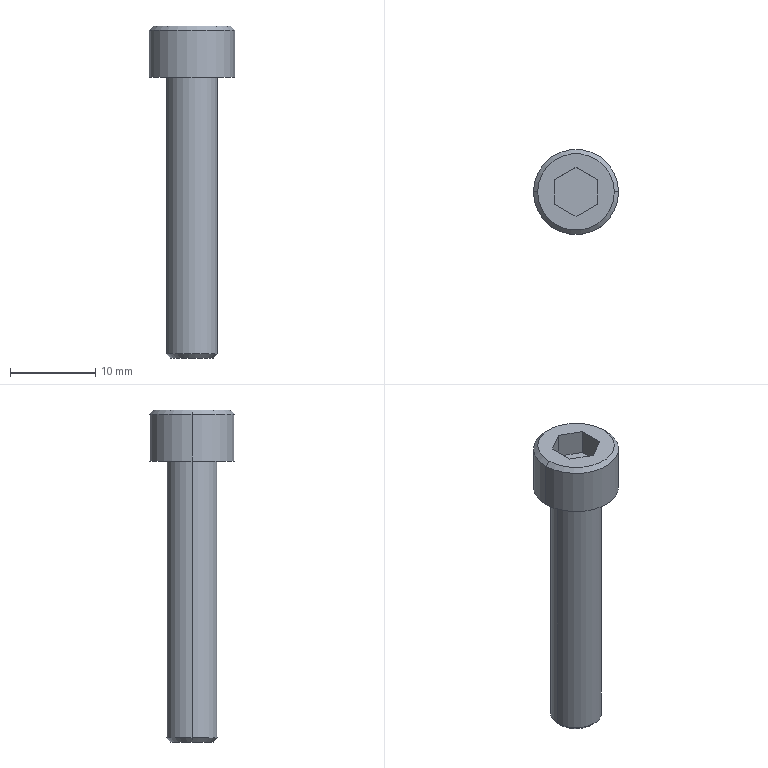Part | Creo | 1 solid | 18 faces | box 10 x 10 x 39 mm | volume 1333 mm3 | plane 10 | cone 4 | cylinder 4 | commonest cylinder face diameters 6 x2 10 x2
STEP:
#1=CARTESIAN_POINT('',(-45.5,235.,-211.5));
#2=VERTEX_POINT('',#1);
#3=CARTESIAN_POINT('',(-54.5,235.,-211.5));
#4=VERTEX_POINT('',#3);
#5=CARTESIAN_POINT('',(-50.,235.,-211.5));
#6=DIRECTION('',(0.,0.,1.));
#7=DIRECTION('',(1.,0.,0.));
#8=AXIS2_PLACEMENT_3D('',#5,#6,#7);
#9=CIRCLE('',#8,4.5);
#10=EDGE_CURVE('',#2,#4,#9,.T.);
#11=ORIENTED_EDGE('',*,*,#10,.F.);
#12=CARTESIAN_POINT('',(-50.,235.,-211.5));
#13=DIRECTION('',(0.,0.,1.));
#14=DIRECTION('',(-1.,0.,0.));
#15=AXIS2_PLACEMENT_3D('',#12,#13,#14);
#16=CIRCLE('',#15,4.5);
#17=EDGE_CURVE('',#4,#2,#16,.T.);
#18=ORIENTED_EDGE('',*,*,#17,.F.);
#19=EDGE_LOOP('',(#11,#18));
#20=FACE_OUTER_BOUND('',#19,.F.);
#21=CARTESIAN_POINT('',(-52.5,233.557,-211.5));
#22=VERTEX_POINT('',#21);
#23=CARTESIAN_POINT('',(-52.5,236.443,-211.5));
#24=VERTEX_POINT('',#23);
#25=CARTESIAN_POINT('',(-52.5,233.557,-211.5));
#26=DIRECTION('',(0.,1.,0.));
#27=VECTOR('',#26,2.887);
#28=LINE('',#25,#27);
#29=EDGE_CURVE('',#22,#24,#28,.T.);
#30=ORIENTED_EDGE('',*,*,#29,.F.);
#31=CARTESIAN_POINT('',(-50.,232.113,-211.5));
#32=VERTEX_POINT('',#31);
#33=CARTESIAN_POINT('',(-50.,232.113,-211.5));
#34=DIRECTION('',(-0.866,0.5,0.));
#35=VECTOR('',#34,2.887);
#36=LINE('',#33,#35);
#37=EDGE_CURVE('',#32,#22,#36,.T.);
#38=ORIENTED_EDGE('',*,*,#37,.F.);
#39=CARTESIAN_POINT('',(-47.5,233.557,-211.5));
#40=VERTEX_POINT('',#39);
#41=CARTESIAN_POINT('',(-47.5,233.557,-211.5));
#42=DIRECTION('',(-0.866,-0.5,0.));
#43=VECTOR('',#42,2.887);
#44=LINE('',#41,#43);
#45=EDGE_CURVE('',#40,#32,#44,.T.);
#46=ORIENTED_EDGE('',*,*,#45,.F.);
#47=CARTESIAN_POINT('',(-47.5,236.443,-211.5));
#48=VERTEX_POINT('',#47);
#49=CARTESIAN_POINT('',(-47.5,236.443,-211.5));
#50=DIRECTION('',(0.,-1.,0.));
#51=VECTOR('',#50,2.887);
#52=LINE('',#49,#51);
#53=EDGE_CURVE('',#48,#40,#52,.T.);
#54=ORIENTED_EDGE('',*,*,#53,.F.);
#55=CARTESIAN_POINT('',(-50.,237.887,-211.5));
#56=VERTEX_POINT('',#55);
#57=CARTESIAN_POINT('',(-50.,237.887,-211.5));
#58=DIRECTION('',(0.866,-0.5,0.));
#59=VECTOR('',#58,2.887);
#60=LINE('',#57,#59);
#61=EDGE_CURVE('',#56,#48,#60,.T.);
#62=ORIENTED_EDGE('',*,*,#61,.F.);
#63=CARTESIAN_POINT('',(-52.5,236.443,-211.5));
#64=DIRECTION('',(0.866,0.5,0.));
#65=VECTOR('',#64,2.887);
#66=LINE('',#63,#65);
#67=EDGE_CURVE('',#24,#56,#66,.T.);
#68=ORIENTED_EDGE('',*,*,#67,.F.);
#69=EDGE_LOOP('',(#30,#38,#46,#54,#62,#68));
#70=FACE_BOUND('',#69,.F.);
#71=CARTESIAN_POINT('',(-50.,235.,-211.5));
#72=DIRECTION('',(0.,0.,1.));
#73=DIRECTION('',(1.,0.,0.));
#74=AXIS2_PLACEMENT_3D('',#71,#72,#73);
#75=PLANE('',#74);
#76=ADVANCED_FACE('',(#20,#70),#75,.T.);
#77=ORIENTED_EDGE('',*,*,#10,.T.);
#78=CARTESIAN_POINT('',(-55.,235.,-212.));
#79=VERTEX_POINT('',#78);
#80=CARTESIAN_POINT('',(-54.5,235.,-211.5));
#81=DIRECTION('',(-0.7071,0.,-0.7071));
#82=VECTOR('',#81,0.7071);
#83=LINE('',#80,#82);
#84=EDGE_CURVE('',#4,#79,#83,.T.);
#85=ORIENTED_EDGE('',*,*,#84,.T.);
#86=CARTESIAN_POINT('',(-45.,235.,-212.));
#87=VERTEX_POINT('',#86);
#88=CARTESIAN_POINT('',(-50.,235.,-212.));
#89=DIRECTION('',(0.,0.,1.));
#90=DIRECTION('',(1.,0.,0.));
#91=AXIS2_PLACEMENT_3D('',#88,#89,#90);
#92=CIRCLE('',#91,5.);
#93=EDGE_CURVE('',#87,#79,#92,.T.);
#94=ORIENTED_EDGE('',*,*,#93,.F.);
#95=CARTESIAN_POINT('',(-45.5,235.,-211.5));
#96=DIRECTION('',(0.7071,0.,-0.7071));
#97=VECTOR('',#96,0.7071);
#98=LINE('',#95,#97);
#99=EDGE_CURVE('',#2,#87,#98,.T.);
#100=ORIENTED_EDGE('',*,*,#99,.F.);
#101=EDGE_LOOP('',(#77,#85,#94,#100));
#102=FACE_OUTER_BOUND('',#101,.F.);
#103=CARTESIAN_POINT('',(-50.,235.,-211.75));
#104=DIRECTION('',(0.,0.,-1.));
#105=DIRECTION('',(-1.,0.,0.));
#106=AXIS2_PLACEMENT_3D('',#103,#104,#105);
#107=CONICAL_SURFACE('',#106,4.75,45.);
#108=ADVANCED_FACE('',(#102),#107,.T.);
#109=ORIENTED_EDGE('',*,*,#17,.T.);
#110=ORIENTED_EDGE('',*,*,#99,.T.);
#111=CARTESIAN_POINT('',(-50.,235.,-212.));
#112=DIRECTION('',(0.,0.,1.));
#113=DIRECTION('',(-1.,0.,0.));
#114=AXIS2_PLACEMENT_3D('',#111,#112,#113);
#115=CIRCLE('',#114,5.);
#116=EDGE_CURVE('',#79,#87,#115,.T.);
#117=ORIENTED_EDGE('',*,*,#116,.F.);
#118=ORIENTED_EDGE('',*,*,#84,.F.);
#119=EDGE_LOOP('',(#109,#110,#117,#118));
#120=FACE_OUTER_BOUND('',#119,.F.);
#121=CARTESIAN_POINT('',(-50.,235.,-211.75));
#122=DIRECTION('',(0.,0.,-1.));
#123=DIRECTION('',(-1.,0.,0.));
#124=AXIS2_PLACEMENT_3D('',#121,#122,#123);
#125=CONICAL_SURFACE('',#124,4.75,45.);
#126=ADVANCED_FACE('',(#120),#125,.T.);
#127=ORIENTED_EDGE('',*,*,#116,.T.);
#128=CARTESIAN_POINT('',(-45.,235.,-217.5));
#129=VERTEX_POINT('',#128);
#130=CARTESIAN_POINT('',(-45.,235.,-217.5));
#131=DIRECTION('',(0.,0.,1.));
#132=VECTOR('',#131,5.5);
#133=LINE('',#130,#132);
#134=EDGE_CURVE('',#129,#87,#133,.T.);
#135=ORIENTED_EDGE('',*,*,#134,.F.);
#136=CARTESIAN_POINT('',(-55.,235.,-217.5));
#137=VERTEX_POINT('',#136);
#138=CARTESIAN_POINT('',(-50.,235.,-217.5));
#139=DIRECTION('',(0.,0.,-1.));
#140=DIRECTION('',(1.,0.,0.));
#141=AXIS2_PLACEMENT_3D('',#138,#139,#140);
#142=CIRCLE('',#141,5.);
#143=EDGE_CURVE('',#129,#137,#142,.T.);
#144=ORIENTED_EDGE('',*,*,#143,.T.);
#145=CARTESIAN_POINT('',(-55.,235.,-217.5));
#146=DIRECTION('',(0.,0.,1.));
#147=VECTOR('',#146,5.5);
#148=LINE('',#145,#147);
#149=EDGE_CURVE('',#137,#79,#148,.T.);
#150=ORIENTED_EDGE('',*,*,#149,.T.);
#151=EDGE_LOOP('',(#127,#135,#144,#150));
#152=FACE_OUTER_BOUND('',#151,.F.);
#153=CARTESIAN_POINT('',(-50.,235.,-217.5));
#154=DIRECTION('',(0.,0.,1.));
#155=DIRECTION('',(1.,0.,0.));
#156=AXIS2_PLACEMENT_3D('',#153,#154,#155);
#157=CYLINDRICAL_SURFACE('',#156,5.);
#158=ADVANCED_FACE('',(#152),#157,.T.);
#159=ORIENTED_EDGE('',*,*,#93,.T.);
#160=ORIENTED_EDGE('',*,*,#149,.F.);
#161=CARTESIAN_POINT('',(-50.,235.,-217.5));
#162=DIRECTION('',(0.,0.,-1.));
#163=DIRECTION('',(-1.,0.,0.));
#164=AXIS2_PLACEMENT_3D('',#161,#162,#163);
#165=CIRCLE('',#164,5.);
#166=EDGE_CURVE('',#137,#129,#165,.T.);
#167=ORIENTED_EDGE('',*,*,#166,.T.);
#168=ORIENTED_EDGE('',*,*,#134,.T.);
#169=EDGE_LOOP('',(#159,#160,#167,#168));
#170=FACE_OUTER_BOUND('',#169,.F.);
#171=CARTESIAN_POINT('',(-50.,235.,-217.5));
#172=DIRECTION('',(0.,0.,1.));
#173=DIRECTION('',(1.,0.,0.));
#174=AXIS2_PLACEMENT_3D('',#171,#172,#173);
#175=CYLINDRICAL_SURFACE('',#174,5.);
#176=ADVANCED_FACE('',(#170),#175,.T.);
#177=ORIENTED_EDGE('',*,*,#143,.F.);
#178=ORIENTED_EDGE('',*,*,#166,.F.);
#179=EDGE_LOOP('',(#177,#178));
#180=FACE_OUTER_BOUND('',#179,.F.);
#181=CARTESIAN_POINT('',(-53.,235.,-217.5));
#182=VERTEX_POINT('',#181);
#183=CARTESIAN_POINT('',(-47.,235.,-217.5));
#184=VERTEX_POINT('',#183);
#185=CARTESIAN_POINT('',(-50.,235.,-217.5));
#186=DIRECTION('',(0.,0.,1.));
#187=DIRECTION('',(-1.,0.,0.));
#188=AXIS2_PLACEMENT_3D('',#185,#186,#187);
#189=CIRCLE('',#188,3.);
#190=EDGE_CURVE('',#182,#184,#189,.T.);
#191=ORIENTED_EDGE('',*,*,#190,.F.);
#192=CARTESIAN_POINT('',(-50.,235.,-217.5));
#193=DIRECTION('',(0.,0.,1.));
#194=DIRECTION('',(1.,0.,0.));
#195=AXIS2_PLACEMENT_3D('',#192,#193,#194);
#196=CIRCLE('',#195,3.);
#197=EDGE_CURVE('',#184,#182,#196,.T.);
#198=ORIENTED_EDGE('',*,*,#197,.F.);
#199=EDGE_LOOP('',(#191,#198));
#200=FACE_BOUND('',#199,.F.);
#201=CARTESIAN_POINT('',(-50.,235.,-217.5));
#202=DIRECTION('',(0.,0.,-1.));
#203=DIRECTION('',(-1.,0.,0.));
#204=AXIS2_PLACEMENT_3D('',#201,#202,#203);
#205=PLANE('',#204);
#206=ADVANCED_FACE('',(#180,#200),#205,.T.);
#207=CARTESIAN_POINT('',(-47.,235.,-250.));
#208=VERTEX_POINT('',#207);
#209=CARTESIAN_POINT('',(-53.,235.,-250.));
#210=VERTEX_POINT('',#209);
#211=CARTESIAN_POINT('',(-50.,235.,-250.));
#212=DIRECTION('',(0.,0.,-1.));
#213=DIRECTION('',(1.,0.,0.));
#214=AXIS2_PLACEMENT_3D('',#211,#212,#213);
#215=CIRCLE('',#214,3.);
#216=EDGE_CURVE('',#208,#210,#215,.T.);
#217=ORIENTED_EDGE('',*,*,#216,.T.);
#218=CARTESIAN_POINT('',(-53.,235.,-217.5));
#219=DIRECTION('',(0.,0.,-1.));
#220=VECTOR('',#219,32.5);
#221=LINE('',#218,#220);
#222=EDGE_CURVE('',#182,#210,#221,.T.);
#223=ORIENTED_EDGE('',*,*,#222,.F.);
#224=ORIENTED_EDGE('',*,*,#190,.T.);
#225=CARTESIAN_POINT('',(-47.,235.,-217.5));
#226=DIRECTION('',(0.,0.,-1.));
#227=VECTOR('',#226,32.5);
#228=LINE('',#225,#227);
#229=EDGE_CURVE('',#184,#208,#228,.T.);
#230=ORIENTED_EDGE('',*,*,#229,.T.);
#231=EDGE_LOOP('',(#217,#223,#224,#230));
#232=FACE_OUTER_BOUND('',#231,.F.);
#233=CARTESIAN_POINT('',(-50.,235.,-217.5));
#234=DIRECTION('',(0.,0.,-1.));
#235=DIRECTION('',(-1.,0.,0.));
#236=AXIS2_PLACEMENT_3D('',#233,#234,#235);
#237=CYLINDRICAL_SURFACE('',#236,3.);
#238=ADVANCED_FACE('',(#232),#237,.T.);
#239=CARTESIAN_POINT('',(-47.5,235.,-250.5));
#240=VERTEX_POINT('',#239);
#241=CARTESIAN_POINT('',(-52.5,235.,-250.5));
#242=VERTEX_POINT('',#241);
#243=CARTESIAN_POINT('',(-50.,235.,-250.5));
#244=DIRECTION('',(0.,0.,-1.));
#245=DIRECTION('',(1.,0.,0.));
#246=AXIS2_PLACEMENT_3D('',#243,#244,#245);
#247=CIRCLE('',#246,2.5);
#248=EDGE_CURVE('',#240,#242,#247,.T.);
#249=ORIENTED_EDGE('',*,*,#248,.T.);
#250=CARTESIAN_POINT('',(-52.5,235.,-250.5));
#251=DIRECTION('',(-0.7071,0.,0.7071));
#252=VECTOR('',#251,0.7071);
#253=LINE('',#250,#252);
#254=EDGE_CURVE('',#242,#210,#253,.T.);
#255=ORIENTED_EDGE('',*,*,#254,.T.);
#256=ORIENTED_EDGE('',*,*,#216,.F.);
#257=CARTESIAN_POINT('',(-47.5,235.,-250.5));
#258=DIRECTION('',(0.7071,0.,0.7071));
#259=VECTOR('',#258,0.7071);
#260=LINE('',#257,#259);
#261=EDGE_CURVE('',#240,#208,#260,.T.);
#262=ORIENTED_EDGE('',*,*,#261,.F.);
#263=EDGE_LOOP('',(#249,#255,#256,#262));
#264=FACE_OUTER_BOUND('',#263,.F.);
#265=CARTESIAN_POINT('',(-50.,235.,-250.25));
#266=DIRECTION('',(0.,0.,1.));
#267=DIRECTION('',(1.,0.,0.));
#268=AXIS2_PLACEMENT_3D('',#265,#266,#267);
#269=CONICAL_SURFACE('',#268,2.75,45.);
#270=ADVANCED_FACE('',(#264),#269,.T.);
#271=CARTESIAN_POINT('',(-50.,235.,-250.5));
#272=DIRECTION('',(0.,0.,-1.));
#273=DIRECTION('',(-1.,0.,0.));
#274=AXIS2_PLACEMENT_3D('',#271,#272,#273);
#275=CIRCLE('',#274,2.5);
#276=EDGE_CURVE('',#242,#240,#275,.T.);
#277=ORIENTED_EDGE('',*,*,#276,.F.);
#278=ORIENTED_EDGE('',*,*,#248,.F.);
#279=EDGE_LOOP('',(#277,#278));
#280=FACE_OUTER_BOUND('',#279,.F.);
#281=CARTESIAN_POINT('',(-50.,235.,-250.5));
#282=DIRECTION('',(0.,0.,-1.));
#283=DIRECTION('',(-1.,0.,0.));
#284=AXIS2_PLACEMENT_3D('',#281,#282,#283);
#285=PLANE('',#284);
#286=ADVANCED_FACE('',(#280),#285,.T.);
#287=ORIENTED_EDGE('',*,*,#276,.T.);
#288=ORIENTED_EDGE('',*,*,#261,.T.);
#289=CARTESIAN_POINT('',(-50.,235.,-250.));
#290=DIRECTION('',(0.,0.,-1.));
#291=DIRECTION('',(-1.,0.,0.));
#292=AXIS2_PLACEMENT_3D('',#289,#290,#291);
#293=CIRCLE('',#292,3.);
#294=EDGE_CURVE('',#210,#208,#293,.T.);
#295=ORIENTED_EDGE('',*,*,#294,.F.);
#296=ORIENTED_EDGE('',*,*,#254,.F.);
#297=EDGE_LOOP('',(#287,#288,#295,#296));
#298=FACE_OUTER_BOUND('',#297,.F.);
#299=CARTESIAN_POINT('',(-50.,235.,-250.25));
#300=DIRECTION('',(0.,0.,1.));
#301=DIRECTION('',(1.,0.,0.));
#302=AXIS2_PLACEMENT_3D('',#299,#300,#301);
#303=CONICAL_SURFACE('',#302,2.75,45.);
#304=ADVANCED_FACE('',(#298),#303,.T.);
#305=ORIENTED_EDGE('',*,*,#294,.T.);
#306=ORIENTED_EDGE('',*,*,#229,.F.);
#307=ORIENTED_EDGE('',*,*,#197,.T.);
#308=ORIENTED_EDGE('',*,*,#222,.T.);
#309=EDGE_LOOP('',(#305,#306,#307,#308));
#310=FACE_OUTER_BOUND('',#309,.F.);
#311=CARTESIAN_POINT('',(-50.,235.,-217.5));
#312=DIRECTION('',(0.,0.,-1.));
#313=DIRECTION('',(-1.,0.,0.));
#314=AXIS2_PLACEMENT_3D('',#311,#312,#313);
#315=CYLINDRICAL_SURFACE('',#314,3.);
#316=ADVANCED_FACE('',(#310),#315,.T.);
#317=ORIENTED_EDGE('',*,*,#29,.T.);
#318=CARTESIAN_POINT('',(-52.5,236.443,-214.5));
#319=VERTEX_POINT('',#318);
#320=CARTESIAN_POINT('',(-52.5,236.443,-211.5));
#321=DIRECTION('',(0.,0.,-1.));
#322=VECTOR('',#321,3.);
#323=LINE('',#320,#322);
#324=EDGE_CURVE('',#24,#319,#323,.T.);
#325=ORIENTED_EDGE('',*,*,#324,.T.);
#326=CARTESIAN_POINT('',(-52.5,233.557,-214.5));
#327=VERTEX_POINT('',#326);
#328=CARTESIAN_POINT('',(-52.5,233.557,-214.5));
#329=DIRECTION('',(0.,1.,0.));
#330=VECTOR('',#329,2.887);
#331=LINE('',#328,#330);
#332=EDGE_CURVE('',#327,#319,#331,.T.);
#333=ORIENTED_EDGE('',*,*,#332,.F.);
#334=CARTESIAN_POINT('',(-52.5,233.557,-211.5));
#335=DIRECTION('',(0.,0.,-1.));
#336=VECTOR('',#335,3.);
#337=LINE('',#334,#336);
#338=EDGE_CURVE('',#22,#327,#337,.T.);
#339=ORIENTED_EDGE('',*,*,#338,.F.);
#340=EDGE_LOOP('',(#317,#325,#333,#339));
#341=FACE_OUTER_BOUND('',#340,.F.);
#342=CARTESIAN_POINT('',(-52.5,235.,-213.));
#343=DIRECTION('',(-1.,0.,0.));
#344=DIRECTION('',(0.,0.,1.));
#345=AXIS2_PLACEMENT_3D('',#342,#343,#344);
#346=PLANE('',#345);
#347=ADVANCED_FACE('',(#341),#346,.F.);
#348=ORIENTED_EDGE('',*,*,#67,.T.);
#349=CARTESIAN_POINT('',(-50.,237.887,-214.5));
#350=VERTEX_POINT('',#349);
#351=CARTESIAN_POINT('',(-50.,237.887,-211.5));
#352=DIRECTION('',(0.,0.,-1.));
#353=VECTOR('',#352,3.);
#354=LINE('',#351,#353);
#355=EDGE_CURVE('',#56,#350,#354,.T.);
#356=ORIENTED_EDGE('',*,*,#355,.T.);
#357=CARTESIAN_POINT('',(-50.,237.887,-214.5));
#358=DIRECTION('',(-0.866,-0.5,0.));
#359=VECTOR('',#358,2.887);
#360=LINE('',#357,#359);
#361=EDGE_CURVE('',#350,#319,#360,.T.);
#362=ORIENTED_EDGE('',*,*,#361,.T.);
#363=ORIENTED_EDGE('',*,*,#324,.F.);
#364=EDGE_LOOP('',(#348,#356,#362,#363));
#365=FACE_OUTER_BOUND('',#364,.F.);
#366=CARTESIAN_POINT('',(-51.25,237.165,-213.));
#367=DIRECTION('',(-0.5,0.866,0.));
#368=DIRECTION('',(-0.866,-0.5,0.));
#369=AXIS2_PLACEMENT_3D('',#366,#367,#368);
#370=PLANE('',#369);
#371=ADVANCED_FACE('',(#365),#370,.F.);
#372=ORIENTED_EDGE('',*,*,#61,.T.);
#373=CARTESIAN_POINT('',(-47.5,236.443,-214.5));
#374=VERTEX_POINT('',#373);
#375=CARTESIAN_POINT('',(-47.5,236.443,-211.5));
#376=DIRECTION('',(0.,0.,-1.));
#377=VECTOR('',#376,3.);
#378=LINE('',#375,#377);
#379=EDGE_CURVE('',#48,#374,#378,.T.);
#380=ORIENTED_EDGE('',*,*,#379,.T.);
#381=CARTESIAN_POINT('',(-47.5,236.443,-214.5));
#382=DIRECTION('',(-0.866,0.5,0.));
#383=VECTOR('',#382,2.887);
#384=LINE('',#381,#383);
#385=EDGE_CURVE('',#374,#350,#384,.T.);
#386=ORIENTED_EDGE('',*,*,#385,.T.);
#387=ORIENTED_EDGE('',*,*,#355,.F.);
#388=EDGE_LOOP('',(#372,#380,#386,#387));
#389=FACE_OUTER_BOUND('',#388,.F.);
#390=CARTESIAN_POINT('',(-48.75,237.165,-213.));
#391=DIRECTION('',(0.5,0.866,0.));
#392=DIRECTION('',(-0.866,0.5,0.));
#393=AXIS2_PLACEMENT_3D('',#390,#391,#392);
#394=PLANE('',#393);
#395=ADVANCED_FACE('',(#389),#394,.F.);
#396=ORIENTED_EDGE('',*,*,#53,.T.);
#397=CARTESIAN_POINT('',(-47.5,233.557,-214.5));
#398=VERTEX_POINT('',#397);
#399=CARTESIAN_POINT('',(-47.5,233.557,-211.5));
#400=DIRECTION('',(0.,0.,-1.));
#401=VECTOR('',#400,3.);
#402=LINE('',#399,#401);
#403=EDGE_CURVE('',#40,#398,#402,.T.);
#404=ORIENTED_EDGE('',*,*,#403,.T.);
#405=CARTESIAN_POINT('',(-47.5,236.443,-214.5));
#406=DIRECTION('',(0.,-1.,0.));
#407=VECTOR('',#406,2.887);
#408=LINE('',#405,#407);
#409=EDGE_CURVE('',#374,#398,#408,.T.);
#410=ORIENTED_EDGE('',*,*,#409,.F.);
#411=ORIENTED_EDGE('',*,*,#379,.F.);
#412=EDGE_LOOP('',(#396,#404,#410,#411));
#413=FACE_OUTER_BOUND('',#412,.F.);
#414=CARTESIAN_POINT('',(-47.5,235.,-213.));
#415=DIRECTION('',(1.,0.,0.));
#416=DIRECTION('',(0.,0.,-1.));
#417=AXIS2_PLACEMENT_3D('',#414,#415,#416);
#418=PLANE('',#417);
#419=ADVANCED_FACE('',(#413),#418,.F.);
#420=ORIENTED_EDGE('',*,*,#45,.T.);
#421=CARTESIAN_POINT('',(-50.,232.113,-214.5));
#422=VERTEX_POINT('',#421);
#423=CARTESIAN_POINT('',(-50.,232.113,-211.5));
#424=DIRECTION('',(0.,0.,-1.));
#425=VECTOR('',#424,3.);
#426=LINE('',#423,#425);
#427=EDGE_CURVE('',#32,#422,#426,.T.);
#428=ORIENTED_EDGE('',*,*,#427,.T.);
#429=CARTESIAN_POINT('',(-50.,232.113,-214.5));
#430=DIRECTION('',(0.866,0.5,0.));
#431=VECTOR('',#430,2.887);
#432=LINE('',#429,#431);
#433=EDGE_CURVE('',#422,#398,#432,.T.);
#434=ORIENTED_EDGE('',*,*,#433,.T.);
#435=ORIENTED_EDGE('',*,*,#403,.F.);
#436=EDGE_LOOP('',(#420,#428,#434,#435));
#437=FACE_OUTER_BOUND('',#436,.F.);
#438=CARTESIAN_POINT('',(-48.75,232.835,-213.));
#439=DIRECTION('',(0.5,-0.866,0.));
#440=DIRECTION('',(0.866,0.5,0.));
#441=AXIS2_PLACEMENT_3D('',#438,#439,#440);
#442=PLANE('',#441);
#443=ADVANCED_FACE('',(#437),#442,.F.);
#444=ORIENTED_EDGE('',*,*,#37,.T.);
#445=ORIENTED_EDGE('',*,*,#338,.T.);
#446=CARTESIAN_POINT('',(-52.5,233.557,-214.5));
#447=DIRECTION('',(0.866,-0.5,0.));
#448=VECTOR('',#447,2.887);
#449=LINE('',#446,#448);
#450=EDGE_CURVE('',#327,#422,#449,.T.);
#451=ORIENTED_EDGE('',*,*,#450,.T.);
#452=ORIENTED_EDGE('',*,*,#427,.F.);
#453=EDGE_LOOP('',(#444,#445,#451,#452));
#454=FACE_OUTER_BOUND('',#453,.F.);
#455=CARTESIAN_POINT('',(-51.25,232.835,-213.));
#456=DIRECTION('',(-0.5,-0.866,0.));
#457=DIRECTION('',(0.866,-0.5,0.));
#458=AXIS2_PLACEMENT_3D('',#455,#456,#457);
#459=PLANE('',#458);
#460=ADVANCED_FACE('',(#454),#459,.F.);
#461=ORIENTED_EDGE('',*,*,#433,.F.);
#462=ORIENTED_EDGE('',*,*,#450,.F.);
#463=ORIENTED_EDGE('',*,*,#332,.T.);
#464=ORIENTED_EDGE('',*,*,#361,.F.);
#465=ORIENTED_EDGE('',*,*,#385,.F.);
#466=ORIENTED_EDGE('',*,*,#409,.T.);
#467=EDGE_LOOP('',(#461,#462,#463,#464,#465,#466));
#468=FACE_OUTER_BOUND('',#467,.F.);
#469=CARTESIAN_POINT('',(-50.,235.,-214.5));
#470=DIRECTION('',(0.,0.,-1.));
#471=DIRECTION('',(-1.,0.,0.));
#472=AXIS2_PLACEMENT_3D('',#469,#470,#471);
#473=PLANE('',#472);
#474=ADVANCED_FACE('',(#468),#473,.F.);
#475=CLOSED_SHELL('',(#76,#108,#126,#158,#176,#206,#238,#270,#286,#304,#316,#347,#371,#395,#419,#443,#460,#474));
#476=MANIFOLD_SOLID_BREP('',#475);
#477=(LENGTH_UNIT()NAMED_UNIT(*)SI_UNIT(.MILLI.,.METRE.));
#478=UNCERTAINTY_MEASURE_WITH_UNIT(LENGTH_MEASURE(0.004148),#477,'','');
#479=(NAMED_UNIT(*)PLANE_ANGLE_UNIT()SI_UNIT($,.RADIAN.));
#480=PLANE_ANGLE_MEASURE_WITH_UNIT(PLANE_ANGLE_MEASURE(0.01745),#479);
#481=(CONVERSION_BASED_UNIT('DEGREE',#480)NAMED_UNIT(*)PLANE_ANGLE_UNIT());
#482=(NAMED_UNIT(*)SI_UNIT($,.STERADIAN.)SOLID_ANGLE_UNIT());
#483=(GEOMETRIC_REPRESENTATION_CONTEXT(3)GLOBAL_UNCERTAINTY_ASSIGNED_CONTEXT((#478))GLOBAL_UNIT_ASSIGNED_CONTEXT((#477,#481,#482))REPRESENTATION_CONTEXT('',''));
#484=ADVANCED_BREP_SHAPE_REPRESENTATION('',(#476),#483);